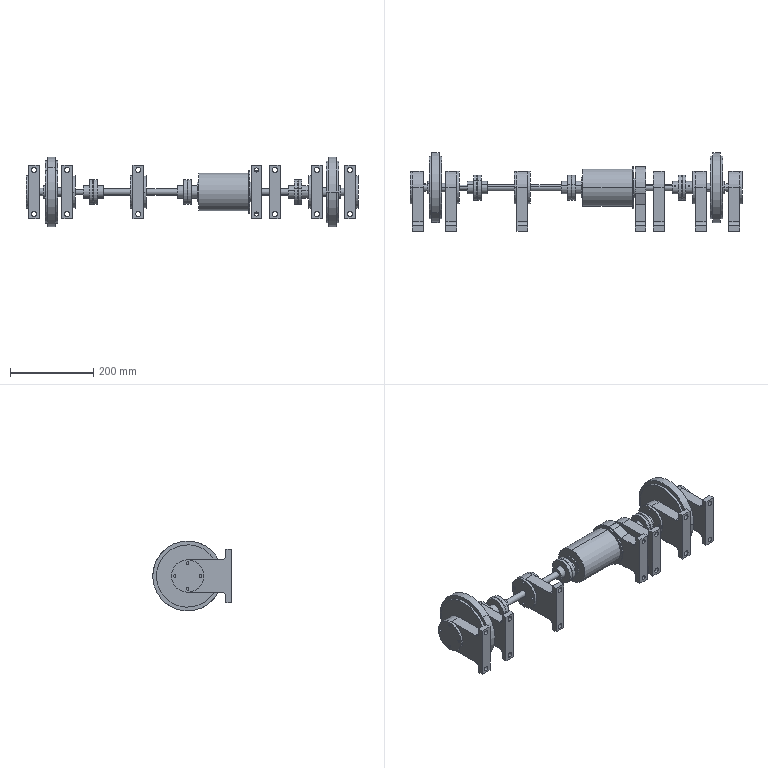Part | NX | features BREP 27 | 94 solids | 904 faces | box 798 x 189 x 168 mm | volume 4416361 mm3 | cylinder 415 | sphere 220 | plane 207 | cone 32 | torus 30 | commonest cylinder face diameters 6 x108 12 x46 36 x36 20 x34 15 x33 28 x20